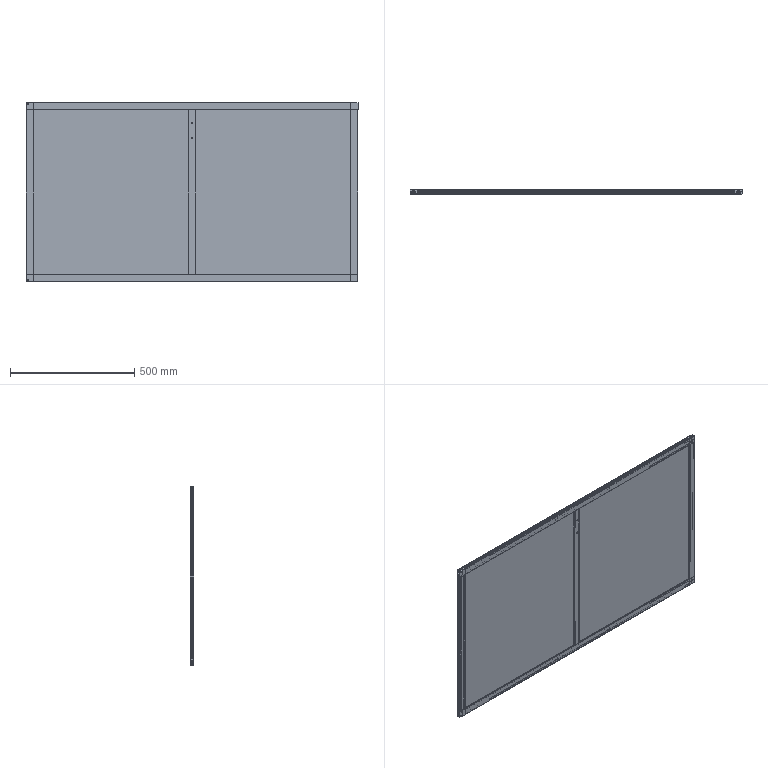Part | SolidWorks | features ReferencePattern 3, LocalLPattern 2 | 19 solids | 893 faces | box 1336 x 15 x 720 mm | volume 5449315 mm3 | plane 570 | cylinder 231 | spline 52 | cone 40 | commonest cylinder face diameters 5 x77 11 x52 1 x42 2 x20 6 x16 6.5 x16